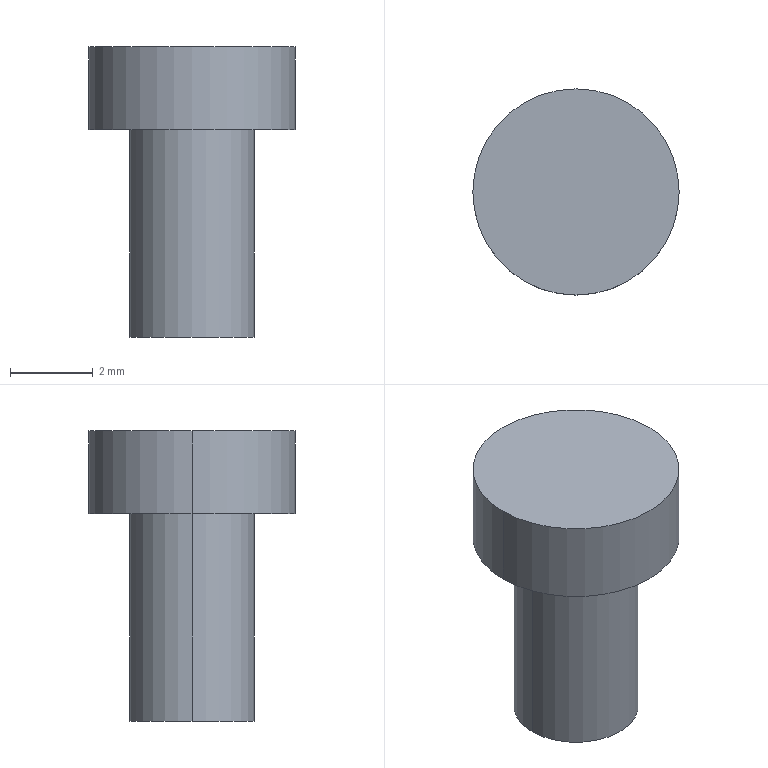Part | SolidWorks | features Extrusion 1, ICE 1 | 1 solid | 7 faces | box 4.973 x 4.973 x 7 mm | volume 74.187 mm3 | cylinder 4 | plane 3 | commonest cylinder face diameters 3 x2 4.973 x2
STEP:
#1=CARTESIAN_POINT('',(-42.711,32.026,2.));
#2=VERTEX_POINT('',#1);
#3=CARTESIAN_POINT('',(-47.684,32.026,2.));
#4=VERTEX_POINT('',#3);
#5=CARTESIAN_POINT('',(-45.198,32.026,2.));
#6=DIRECTION('',(0.,0.,1.));
#7=DIRECTION('',(1.,0.,0.));
#8=AXIS2_PLACEMENT_3D('',#5,#6,#7);
#9=CIRCLE('',#8,2.486);
#10=EDGE_CURVE('',#2,#4,#9,.T.);
#11=ORIENTED_EDGE('',*,*,#10,.F.);
#12=CARTESIAN_POINT('',(-42.711,32.026,0.));
#13=VERTEX_POINT('',#12);
#14=CARTESIAN_POINT('',(-42.711,32.026,2.));
#15=DIRECTION('',(0.,0.,-1.));
#16=VECTOR('',#15,1000.);
#17=LINE('',#14,#16);
#18=EDGE_CURVE('',#2,#13,#17,.T.);
#19=ORIENTED_EDGE('',*,*,#18,.T.);
#20=CARTESIAN_POINT('',(-47.684,32.026,0.));
#21=VERTEX_POINT('',#20);
#22=CARTESIAN_POINT('',(-45.198,32.026,0.));
#23=DIRECTION('',(0.,0.,1.));
#24=DIRECTION('',(1.,0.,0.));
#25=AXIS2_PLACEMENT_3D('',#22,#23,#24);
#26=CIRCLE('',#25,2.486);
#27=EDGE_CURVE('',#13,#21,#26,.T.);
#28=ORIENTED_EDGE('',*,*,#27,.T.);
#29=CARTESIAN_POINT('',(-47.684,32.026,2.));
#30=DIRECTION('',(0.,0.,-1.));
#31=VECTOR('',#30,1000.);
#32=LINE('',#29,#31);
#33=EDGE_CURVE('',#4,#21,#32,.T.);
#34=ORIENTED_EDGE('',*,*,#33,.F.);
#35=EDGE_LOOP('',(#11,#19,#28,#34));
#36=FACE_OUTER_BOUND('',#35,.T.);
#37=CARTESIAN_POINT('',(-45.198,32.026,2.));
#38=DIRECTION('',(0.,0.,-1.));
#39=DIRECTION('',(-1.,0.,0.));
#40=AXIS2_PLACEMENT_3D('',#37,#38,#39);
#41=CYLINDRICAL_SURFACE('',#40,2.486);
#42=ADVANCED_FACE('',(#36),#41,.T.);
#43=CARTESIAN_POINT('',(-43.698,32.026,-5.));
#44=VERTEX_POINT('',#43);
#45=CARTESIAN_POINT('',(-46.698,32.026,-5.));
#46=VERTEX_POINT('',#45);
#47=CARTESIAN_POINT('',(-45.198,32.026,-5.));
#48=DIRECTION('',(0.,0.,1.));
#49=DIRECTION('',(1.,0.,0.));
#50=AXIS2_PLACEMENT_3D('',#47,#48,#49);
#51=CIRCLE('',#50,1.5);
#52=EDGE_CURVE('',#44,#46,#51,.T.);
#53=ORIENTED_EDGE('',*,*,#52,.T.);
#54=CARTESIAN_POINT('',(-46.698,32.026,0.));
#55=VERTEX_POINT('',#54);
#56=CARTESIAN_POINT('',(-46.698,32.026,-5.));
#57=DIRECTION('',(0.,0.,1.));
#58=VECTOR('',#57,1000.);
#59=LINE('',#56,#58);
#60=EDGE_CURVE('',#46,#55,#59,.T.);
#61=ORIENTED_EDGE('',*,*,#60,.T.);
#62=CARTESIAN_POINT('',(-43.698,32.026,0.));
#63=VERTEX_POINT('',#62);
#64=CARTESIAN_POINT('',(-45.198,32.026,0.));
#65=DIRECTION('',(0.,0.,1.));
#66=DIRECTION('',(1.,0.,0.));
#67=AXIS2_PLACEMENT_3D('',#64,#65,#66);
#68=CIRCLE('',#67,1.5);
#69=EDGE_CURVE('',#63,#55,#68,.T.);
#70=ORIENTED_EDGE('',*,*,#69,.F.);
#71=CARTESIAN_POINT('',(-43.698,32.026,-5.));
#72=DIRECTION('',(0.,0.,1.));
#73=VECTOR('',#72,1000.);
#74=LINE('',#71,#73);
#75=EDGE_CURVE('',#44,#63,#74,.T.);
#76=ORIENTED_EDGE('',*,*,#75,.F.);
#77=EDGE_LOOP('',(#53,#61,#70,#76));
#78=FACE_OUTER_BOUND('',#77,.T.);
#79=CARTESIAN_POINT('',(-45.198,32.026,-5.));
#80=DIRECTION('',(0.,0.,1.));
#81=DIRECTION('',(1.,0.,0.));
#82=AXIS2_PLACEMENT_3D('',#79,#80,#81);
#83=CYLINDRICAL_SURFACE('',#82,1.5);
#84=ADVANCED_FACE('',(#78),#83,.T.);
#85=ORIENTED_EDGE('',*,*,#60,.F.);
#86=CARTESIAN_POINT('',(-45.198,32.026,-5.));
#87=DIRECTION('',(0.,0.,1.));
#88=DIRECTION('',(1.,0.,0.));
#89=AXIS2_PLACEMENT_3D('',#86,#87,#88);
#90=CIRCLE('',#89,1.5);
#91=EDGE_CURVE('',#46,#44,#90,.T.);
#92=ORIENTED_EDGE('',*,*,#91,.T.);
#93=ORIENTED_EDGE('',*,*,#75,.T.);
#94=CARTESIAN_POINT('',(-45.198,32.026,0.));
#95=DIRECTION('',(0.,0.,1.));
#96=DIRECTION('',(1.,0.,0.));
#97=AXIS2_PLACEMENT_3D('',#94,#95,#96);
#98=CIRCLE('',#97,1.5);
#99=EDGE_CURVE('',#55,#63,#98,.T.);
#100=ORIENTED_EDGE('',*,*,#99,.F.);
#101=EDGE_LOOP('',(#85,#92,#93,#100));
#102=FACE_OUTER_BOUND('',#101,.T.);
#103=CARTESIAN_POINT('',(-45.198,32.026,-5.));
#104=DIRECTION('',(0.,0.,1.));
#105=DIRECTION('',(1.,0.,0.));
#106=AXIS2_PLACEMENT_3D('',#103,#104,#105);
#107=CYLINDRICAL_SURFACE('',#106,1.5);
#108=ADVANCED_FACE('',(#102),#107,.T.);
#109=ORIENTED_EDGE('',*,*,#52,.F.);
#110=ORIENTED_EDGE('',*,*,#91,.F.);
#111=EDGE_LOOP('',(#109,#110));
#112=FACE_OUTER_BOUND('',#111,.T.);
#113=CARTESIAN_POINT('',(-45.198,32.026,-5.));
#114=DIRECTION('',(0.,0.,1.));
#115=DIRECTION('',(1.,0.,0.));
#116=AXIS2_PLACEMENT_3D('',#113,#114,#115);
#117=PLANE('',#116);
#118=ADVANCED_FACE('',(#112),#117,.F.);
#119=ORIENTED_EDGE('',*,*,#18,.F.);
#120=CARTESIAN_POINT('',(-45.198,32.026,2.));
#121=DIRECTION('',(0.,0.,1.));
#122=DIRECTION('',(1.,0.,0.));
#123=AXIS2_PLACEMENT_3D('',#120,#121,#122);
#124=CIRCLE('',#123,2.486);
#125=EDGE_CURVE('',#4,#2,#124,.T.);
#126=ORIENTED_EDGE('',*,*,#125,.F.);
#127=ORIENTED_EDGE('',*,*,#33,.T.);
#128=CARTESIAN_POINT('',(-45.198,32.026,0.));
#129=DIRECTION('',(0.,0.,1.));
#130=DIRECTION('',(1.,0.,0.));
#131=AXIS2_PLACEMENT_3D('',#128,#129,#130);
#132=CIRCLE('',#131,2.486);
#133=EDGE_CURVE('',#21,#13,#132,.T.);
#134=ORIENTED_EDGE('',*,*,#133,.T.);
#135=EDGE_LOOP('',(#119,#126,#127,#134));
#136=FACE_OUTER_BOUND('',#135,.T.);
#137=CARTESIAN_POINT('',(-45.198,32.026,2.));
#138=DIRECTION('',(0.,0.,-1.));
#139=DIRECTION('',(-1.,0.,0.));
#140=AXIS2_PLACEMENT_3D('',#137,#138,#139);
#141=CYLINDRICAL_SURFACE('',#140,2.486);
#142=ADVANCED_FACE('',(#136),#141,.T.);
#143=ORIENTED_EDGE('',*,*,#125,.T.);
#144=ORIENTED_EDGE('',*,*,#10,.T.);
#145=EDGE_LOOP('',(#143,#144));
#146=FACE_OUTER_BOUND('',#145,.T.);
#147=CARTESIAN_POINT('',(-45.198,32.026,2.));
#148=DIRECTION('',(0.,0.,1.));
#149=DIRECTION('',(1.,0.,0.));
#150=AXIS2_PLACEMENT_3D('',#147,#148,#149);
#151=PLANE('',#150);
#152=ADVANCED_FACE('',(#146),#151,.T.);
#153=ORIENTED_EDGE('',*,*,#69,.T.);
#154=ORIENTED_EDGE('',*,*,#99,.T.);
#155=EDGE_LOOP('',(#153,#154));
#156=FACE_BOUND('',#155,.T.);
#157=ORIENTED_EDGE('',*,*,#133,.F.);
#158=ORIENTED_EDGE('',*,*,#27,.F.);
#159=EDGE_LOOP('',(#157,#158));
#160=FACE_OUTER_BOUND('',#159,.T.);
#161=CARTESIAN_POINT('',(-45.198,32.026,0.));
#162=DIRECTION('',(0.,0.,1.));
#163=DIRECTION('',(1.,0.,0.));
#164=AXIS2_PLACEMENT_3D('',#161,#162,#163);
#165=PLANE('',#164);
#166=ADVANCED_FACE('',(#156,#160),#165,.F.);
#167=CLOSED_SHELL('',(#42,#84,#108,#118,#142,#152,#166));
#168=MANIFOLD_SOLID_BREP('',#167);
#169=CARTESIAN_POINT('',(0.,0.,0.));
#170=DIRECTION('',(0.,0.,1.));
#171=DIRECTION('',(1.,0.,0.));
#172=AXIS2_PLACEMENT_3D('',#169,#170,#171);
#173=(LENGTH_UNIT()NAMED_UNIT(*)SI_UNIT(.MILLI.,.METRE.));
#174=UNCERTAINTY_MEASURE_WITH_UNIT(LENGTH_MEASURE(0.00001),#173,'','');
#175=(NAMED_UNIT(*)PLANE_ANGLE_UNIT()SI_UNIT($,.RADIAN.));
#176=(NAMED_UNIT(*)SI_UNIT($,.STERADIAN.)SOLID_ANGLE_UNIT());
#177=(GEOMETRIC_REPRESENTATION_CONTEXT(3)GLOBAL_UNCERTAINTY_ASSIGNED_CONTEXT((#174))GLOBAL_UNIT_ASSIGNED_CONTEXT((#173,#175,#176))REPRESENTATION_CONTEXT('',''));
#178=ADVANCED_BREP_SHAPE_REPRESENTATION('',(#168,#172),#177);